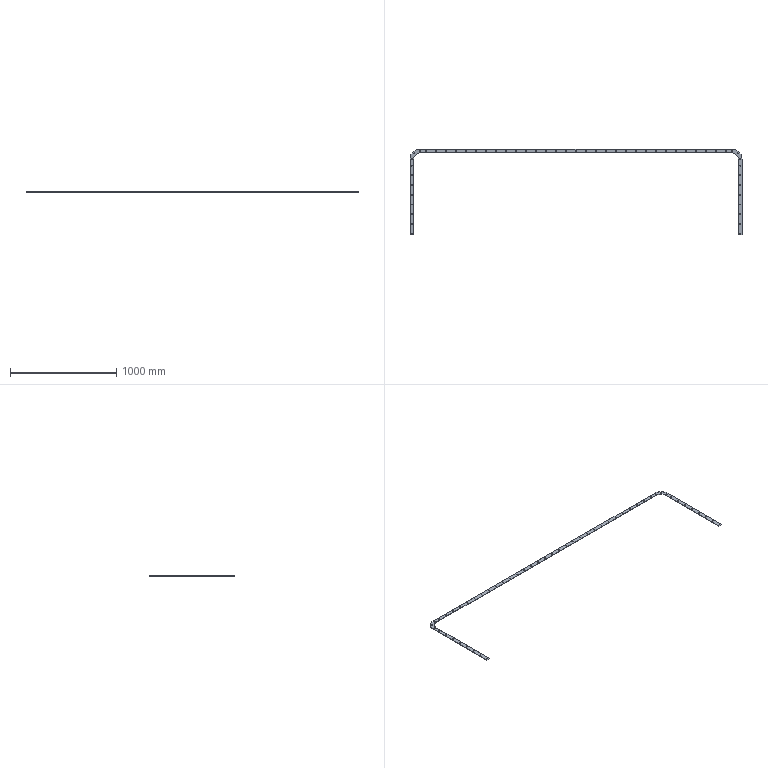Part | SolidWorks | features ICE 3, Extrusion 1 | 1 solid | 226 faces | box 3121 x 804 x 3 mm | volume 477899 mm3 | cylinder 110 | cone 106 | plane 10 | commonest cylinder face diameters 4.5 x106 114 x2 184 x2